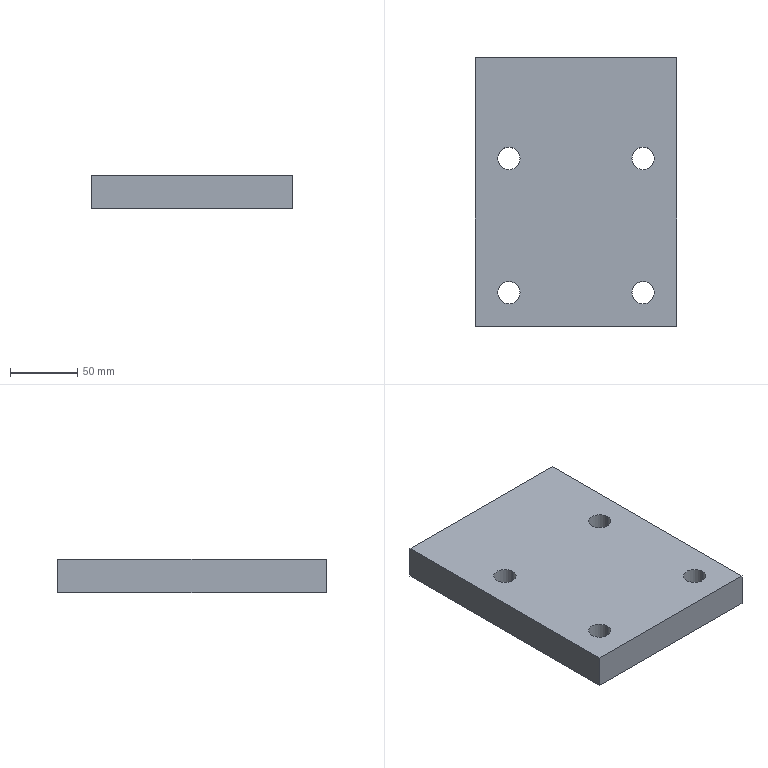Part | SolidWorks | features 3DProfileFeature 1, Extrusion 1, HoleWzd 1 | 1 solid | 14 faces | box 150 x 200 x 25 mm | volume 728181 mm3 | cylinder 8 | plane 6 | commonest cylinder face diameters 16.667 x8
STEP:
#1=CARTESIAN_POINT('',(16.666,125.,0.));
#2=VERTEX_POINT('',#1);
#3=CARTESIAN_POINT('',(33.334,125.,0.));
#4=VERTEX_POINT('',#3);
#5=CARTESIAN_POINT('',(25.,125.,0.));
#6=DIRECTION('',(0.,0.,1.));
#7=DIRECTION('',(1.,0.,0.));
#8=AXIS2_PLACEMENT_3D('',#5,#6,#7);
#9=CIRCLE('',#8,8.334);
#10=EDGE_CURVE('',#2,#4,#9,.T.);
#11=ORIENTED_EDGE('',*,*,#10,.F.);
#12=CARTESIAN_POINT('',(16.666,125.,25.));
#13=VERTEX_POINT('',#12);
#14=CARTESIAN_POINT('',(16.666,125.,25.));
#15=DIRECTION('',(0.,0.,1.));
#16=VECTOR('',#15,1000.);
#17=LINE('',#14,#16);
#18=EDGE_CURVE('',#2,#13,#17,.T.);
#19=ORIENTED_EDGE('',*,*,#18,.T.);
#20=CARTESIAN_POINT('',(33.334,125.,25.));
#21=VERTEX_POINT('',#20);
#22=CARTESIAN_POINT('',(25.,125.,25.));
#23=DIRECTION('',(0.,0.,1.));
#24=DIRECTION('',(1.,0.,0.));
#25=AXIS2_PLACEMENT_3D('',#22,#23,#24);
#26=CIRCLE('',#25,8.334);
#27=EDGE_CURVE('',#13,#21,#26,.T.);
#28=ORIENTED_EDGE('',*,*,#27,.T.);
#29=CARTESIAN_POINT('',(33.334,125.,25.));
#30=DIRECTION('',(0.,0.,1.));
#31=VECTOR('',#30,1000.);
#32=LINE('',#29,#31);
#33=EDGE_CURVE('',#4,#21,#32,.T.);
#34=ORIENTED_EDGE('',*,*,#33,.F.);
#35=EDGE_LOOP('',(#11,#19,#28,#34));
#36=FACE_OUTER_BOUND('',#35,.T.);
#37=CARTESIAN_POINT('',(25.,125.,25.));
#38=DIRECTION('',(0.,0.,1.));
#39=DIRECTION('',(1.,0.,0.));
#40=AXIS2_PLACEMENT_3D('',#37,#38,#39);
#41=CYLINDRICAL_SURFACE('',#40,8.334);
#42=ADVANCED_FACE('',(#36),#41,.F.);
#43=CARTESIAN_POINT('',(116.666,125.,0.));
#44=VERTEX_POINT('',#43);
#45=CARTESIAN_POINT('',(133.334,125.,0.));
#46=VERTEX_POINT('',#45);
#47=CARTESIAN_POINT('',(125.,125.,0.));
#48=DIRECTION('',(0.,0.,1.));
#49=DIRECTION('',(1.,0.,0.));
#50=AXIS2_PLACEMENT_3D('',#47,#48,#49);
#51=CIRCLE('',#50,8.334);
#52=EDGE_CURVE('',#44,#46,#51,.T.);
#53=ORIENTED_EDGE('',*,*,#52,.F.);
#54=CARTESIAN_POINT('',(116.666,125.,25.));
#55=VERTEX_POINT('',#54);
#56=CARTESIAN_POINT('',(116.666,125.,25.));
#57=DIRECTION('',(0.,0.,1.));
#58=VECTOR('',#57,1000.);
#59=LINE('',#56,#58);
#60=EDGE_CURVE('',#44,#55,#59,.T.);
#61=ORIENTED_EDGE('',*,*,#60,.T.);
#62=CARTESIAN_POINT('',(133.334,125.,25.));
#63=VERTEX_POINT('',#62);
#64=CARTESIAN_POINT('',(125.,125.,25.));
#65=DIRECTION('',(0.,0.,1.));
#66=DIRECTION('',(1.,0.,0.));
#67=AXIS2_PLACEMENT_3D('',#64,#65,#66);
#68=CIRCLE('',#67,8.334);
#69=EDGE_CURVE('',#55,#63,#68,.T.);
#70=ORIENTED_EDGE('',*,*,#69,.T.);
#71=CARTESIAN_POINT('',(133.334,125.,25.));
#72=DIRECTION('',(0.,0.,1.));
#73=VECTOR('',#72,1000.);
#74=LINE('',#71,#73);
#75=EDGE_CURVE('',#46,#63,#74,.T.);
#76=ORIENTED_EDGE('',*,*,#75,.F.);
#77=EDGE_LOOP('',(#53,#61,#70,#76));
#78=FACE_OUTER_BOUND('',#77,.T.);
#79=CARTESIAN_POINT('',(125.,125.,25.));
#80=DIRECTION('',(0.,0.,1.));
#81=DIRECTION('',(1.,0.,0.));
#82=AXIS2_PLACEMENT_3D('',#79,#80,#81);
#83=CYLINDRICAL_SURFACE('',#82,8.334);
#84=ADVANCED_FACE('',(#78),#83,.F.);
#85=CARTESIAN_POINT('',(16.666,25.,0.));
#86=VERTEX_POINT('',#85);
#87=CARTESIAN_POINT('',(33.334,25.,0.));
#88=VERTEX_POINT('',#87);
#89=CARTESIAN_POINT('',(25.,25.,0.));
#90=DIRECTION('',(0.,0.,1.));
#91=DIRECTION('',(1.,0.,0.));
#92=AXIS2_PLACEMENT_3D('',#89,#90,#91);
#93=CIRCLE('',#92,8.334);
#94=EDGE_CURVE('',#86,#88,#93,.T.);
#95=ORIENTED_EDGE('',*,*,#94,.F.);
#96=CARTESIAN_POINT('',(16.666,25.,25.));
#97=VERTEX_POINT('',#96);
#98=CARTESIAN_POINT('',(16.666,25.,25.));
#99=DIRECTION('',(0.,0.,1.));
#100=VECTOR('',#99,1000.);
#101=LINE('',#98,#100);
#102=EDGE_CURVE('',#86,#97,#101,.T.);
#103=ORIENTED_EDGE('',*,*,#102,.T.);
#104=CARTESIAN_POINT('',(33.334,25.,25.));
#105=VERTEX_POINT('',#104);
#106=CARTESIAN_POINT('',(25.,25.,25.));
#107=DIRECTION('',(0.,0.,1.));
#108=DIRECTION('',(1.,0.,0.));
#109=AXIS2_PLACEMENT_3D('',#106,#107,#108);
#110=CIRCLE('',#109,8.334);
#111=EDGE_CURVE('',#97,#105,#110,.T.);
#112=ORIENTED_EDGE('',*,*,#111,.T.);
#113=CARTESIAN_POINT('',(33.334,25.,25.));
#114=DIRECTION('',(0.,0.,1.));
#115=VECTOR('',#114,1000.);
#116=LINE('',#113,#115);
#117=EDGE_CURVE('',#88,#105,#116,.T.);
#118=ORIENTED_EDGE('',*,*,#117,.F.);
#119=EDGE_LOOP('',(#95,#103,#112,#118));
#120=FACE_OUTER_BOUND('',#119,.T.);
#121=CARTESIAN_POINT('',(25.,25.,25.));
#122=DIRECTION('',(0.,0.,1.));
#123=DIRECTION('',(1.,0.,0.));
#124=AXIS2_PLACEMENT_3D('',#121,#122,#123);
#125=CYLINDRICAL_SURFACE('',#124,8.334);
#126=ADVANCED_FACE('',(#120),#125,.F.);
#127=CARTESIAN_POINT('',(116.666,25.,0.));
#128=VERTEX_POINT('',#127);
#129=CARTESIAN_POINT('',(133.334,25.,0.));
#130=VERTEX_POINT('',#129);
#131=CARTESIAN_POINT('',(125.,25.,0.));
#132=DIRECTION('',(0.,0.,1.));
#133=DIRECTION('',(1.,0.,0.));
#134=AXIS2_PLACEMENT_3D('',#131,#132,#133);
#135=CIRCLE('',#134,8.334);
#136=EDGE_CURVE('',#128,#130,#135,.T.);
#137=ORIENTED_EDGE('',*,*,#136,.F.);
#138=CARTESIAN_POINT('',(116.666,25.,25.));
#139=VERTEX_POINT('',#138);
#140=CARTESIAN_POINT('',(116.666,25.,25.));
#141=DIRECTION('',(0.,0.,1.));
#142=VECTOR('',#141,1000.);
#143=LINE('',#140,#142);
#144=EDGE_CURVE('',#128,#139,#143,.T.);
#145=ORIENTED_EDGE('',*,*,#144,.T.);
#146=CARTESIAN_POINT('',(133.334,25.,25.));
#147=VERTEX_POINT('',#146);
#148=CARTESIAN_POINT('',(125.,25.,25.));
#149=DIRECTION('',(0.,0.,1.));
#150=DIRECTION('',(1.,0.,0.));
#151=AXIS2_PLACEMENT_3D('',#148,#149,#150);
#152=CIRCLE('',#151,8.334);
#153=EDGE_CURVE('',#139,#147,#152,.T.);
#154=ORIENTED_EDGE('',*,*,#153,.T.);
#155=CARTESIAN_POINT('',(133.334,25.,25.));
#156=DIRECTION('',(0.,0.,1.));
#157=VECTOR('',#156,1000.);
#158=LINE('',#155,#157);
#159=EDGE_CURVE('',#130,#147,#158,.T.);
#160=ORIENTED_EDGE('',*,*,#159,.F.);
#161=EDGE_LOOP('',(#137,#145,#154,#160));
#162=FACE_OUTER_BOUND('',#161,.T.);
#163=CARTESIAN_POINT('',(125.,25.,25.));
#164=DIRECTION('',(0.,0.,1.));
#165=DIRECTION('',(1.,0.,0.));
#166=AXIS2_PLACEMENT_3D('',#163,#164,#165);
#167=CYLINDRICAL_SURFACE('',#166,8.334);
#168=ADVANCED_FACE('',(#162),#167,.F.);
#169=CARTESIAN_POINT('',(25.,125.,0.));
#170=DIRECTION('',(0.,0.,1.));
#171=DIRECTION('',(1.,0.,0.));
#172=AXIS2_PLACEMENT_3D('',#169,#170,#171);
#173=CIRCLE('',#172,8.334);
#174=EDGE_CURVE('',#4,#2,#173,.T.);
#175=ORIENTED_EDGE('',*,*,#174,.T.);
#176=ORIENTED_EDGE('',*,*,#10,.T.);
#177=EDGE_LOOP('',(#175,#176));
#178=FACE_BOUND('',#177,.T.);
#179=CARTESIAN_POINT('',(125.,125.,0.));
#180=DIRECTION('',(0.,0.,1.));
#181=DIRECTION('',(1.,0.,0.));
#182=AXIS2_PLACEMENT_3D('',#179,#180,#181);
#183=CIRCLE('',#182,8.334);
#184=EDGE_CURVE('',#46,#44,#183,.T.);
#185=ORIENTED_EDGE('',*,*,#184,.T.);
#186=ORIENTED_EDGE('',*,*,#52,.T.);
#187=EDGE_LOOP('',(#185,#186));
#188=FACE_BOUND('',#187,.T.);
#189=CARTESIAN_POINT('',(0.,200.,0.));
#190=VERTEX_POINT('',#189);
#191=CARTESIAN_POINT('',(0.,0.,0.));
#192=VERTEX_POINT('',#191);
#193=CARTESIAN_POINT('',(0.,0.,0.));
#194=DIRECTION('',(0.,-1.,0.));
#195=VECTOR('',#194,1000.);
#196=LINE('',#193,#195);
#197=EDGE_CURVE('',#190,#192,#196,.T.);
#198=ORIENTED_EDGE('',*,*,#197,.F.);
#199=CARTESIAN_POINT('',(150.,200.,0.));
#200=VERTEX_POINT('',#199);
#201=CARTESIAN_POINT('',(0.,200.,0.));
#202=DIRECTION('',(-1.,0.,0.));
#203=VECTOR('',#202,1000.);
#204=LINE('',#201,#203);
#205=EDGE_CURVE('',#200,#190,#204,.T.);
#206=ORIENTED_EDGE('',*,*,#205,.F.);
#207=CARTESIAN_POINT('',(150.,0.,0.));
#208=VERTEX_POINT('',#207);
#209=CARTESIAN_POINT('',(150.,0.,0.));
#210=DIRECTION('',(0.,1.,0.));
#211=VECTOR('',#210,1000.);
#212=LINE('',#209,#211);
#213=EDGE_CURVE('',#208,#200,#212,.T.);
#214=ORIENTED_EDGE('',*,*,#213,.F.);
#215=CARTESIAN_POINT('',(0.,0.,0.));
#216=DIRECTION('',(1.,0.,0.));
#217=VECTOR('',#216,1000.);
#218=LINE('',#215,#217);
#219=EDGE_CURVE('',#192,#208,#218,.T.);
#220=ORIENTED_EDGE('',*,*,#219,.F.);
#221=EDGE_LOOP('',(#198,#206,#214,#220));
#222=FACE_OUTER_BOUND('',#221,.T.);
#223=CARTESIAN_POINT('',(125.,25.,0.));
#224=DIRECTION('',(0.,0.,1.));
#225=DIRECTION('',(1.,0.,0.));
#226=AXIS2_PLACEMENT_3D('',#223,#224,#225);
#227=CIRCLE('',#226,8.334);
#228=EDGE_CURVE('',#130,#128,#227,.T.);
#229=ORIENTED_EDGE('',*,*,#228,.T.);
#230=ORIENTED_EDGE('',*,*,#136,.T.);
#231=EDGE_LOOP('',(#229,#230));
#232=FACE_BOUND('',#231,.T.);
#233=CARTESIAN_POINT('',(25.,25.,0.));
#234=DIRECTION('',(0.,0.,1.));
#235=DIRECTION('',(1.,0.,0.));
#236=AXIS2_PLACEMENT_3D('',#233,#234,#235);
#237=CIRCLE('',#236,8.334);
#238=EDGE_CURVE('',#88,#86,#237,.T.);
#239=ORIENTED_EDGE('',*,*,#238,.T.);
#240=ORIENTED_EDGE('',*,*,#94,.T.);
#241=EDGE_LOOP('',(#239,#240));
#242=FACE_BOUND('',#241,.T.);
#243=CARTESIAN_POINT('',(0.,0.,0.));
#244=DIRECTION('',(0.,0.,-1.));
#245=DIRECTION('',(-1.,0.,0.));
#246=AXIS2_PLACEMENT_3D('',#243,#244,#245);
#247=PLANE('',#246);
#248=ADVANCED_FACE('',(#178,#188,#222,#232,#242),#247,.T.);
#249=ORIENTED_EDGE('',*,*,#197,.T.);
#250=CARTESIAN_POINT('',(0.,0.,25.));
#251=VERTEX_POINT('',#250);
#252=CARTESIAN_POINT('',(0.,0.,25.));
#253=DIRECTION('',(0.,0.,-1.));
#254=VECTOR('',#253,1000.);
#255=LINE('',#252,#254);
#256=EDGE_CURVE('',#251,#192,#255,.T.);
#257=ORIENTED_EDGE('',*,*,#256,.F.);
#258=CARTESIAN_POINT('',(0.,200.,25.));
#259=VERTEX_POINT('',#258);
#260=CARTESIAN_POINT('',(0.,0.,25.));
#261=DIRECTION('',(0.,-1.,0.));
#262=VECTOR('',#261,1000.);
#263=LINE('',#260,#262);
#264=EDGE_CURVE('',#259,#251,#263,.T.);
#265=ORIENTED_EDGE('',*,*,#264,.F.);
#266=CARTESIAN_POINT('',(0.,200.,25.));
#267=DIRECTION('',(0.,0.,-1.));
#268=VECTOR('',#267,1000.);
#269=LINE('',#266,#268);
#270=EDGE_CURVE('',#259,#190,#269,.T.);
#271=ORIENTED_EDGE('',*,*,#270,.T.);
#272=EDGE_LOOP('',(#249,#257,#265,#271));
#273=FACE_OUTER_BOUND('',#272,.T.);
#274=CARTESIAN_POINT('',(0.,0.,25.));
#275=DIRECTION('',(1.,0.,0.));
#276=DIRECTION('',(0.,1.,0.));
#277=AXIS2_PLACEMENT_3D('',#274,#275,#276);
#278=PLANE('',#277);
#279=ADVANCED_FACE('',(#273),#278,.F.);
#280=ORIENTED_EDGE('',*,*,#219,.T.);
#281=CARTESIAN_POINT('',(150.,0.,25.));
#282=VERTEX_POINT('',#281);
#283=CARTESIAN_POINT('',(150.,0.,25.));
#284=DIRECTION('',(0.,0.,-1.));
#285=VECTOR('',#284,1000.);
#286=LINE('',#283,#285);
#287=EDGE_CURVE('',#282,#208,#286,.T.);
#288=ORIENTED_EDGE('',*,*,#287,.F.);
#289=CARTESIAN_POINT('',(0.,0.,25.));
#290=DIRECTION('',(1.,0.,0.));
#291=VECTOR('',#290,1000.);
#292=LINE('',#289,#291);
#293=EDGE_CURVE('',#251,#282,#292,.T.);
#294=ORIENTED_EDGE('',*,*,#293,.F.);
#295=ORIENTED_EDGE('',*,*,#256,.T.);
#296=EDGE_LOOP('',(#280,#288,#294,#295));
#297=FACE_OUTER_BOUND('',#296,.T.);
#298=CARTESIAN_POINT('',(0.,0.,25.));
#299=DIRECTION('',(0.,1.,0.));
#300=DIRECTION('',(0.,0.,1.));
#301=AXIS2_PLACEMENT_3D('',#298,#299,#300);
#302=PLANE('',#301);
#303=ADVANCED_FACE('',(#297),#302,.F.);
#304=ORIENTED_EDGE('',*,*,#213,.T.);
#305=CARTESIAN_POINT('',(150.,200.,25.));
#306=VERTEX_POINT('',#305);
#307=CARTESIAN_POINT('',(150.,200.,25.));
#308=DIRECTION('',(0.,0.,-1.));
#309=VECTOR('',#308,1000.);
#310=LINE('',#307,#309);
#311=EDGE_CURVE('',#306,#200,#310,.T.);
#312=ORIENTED_EDGE('',*,*,#311,.F.);
#313=CARTESIAN_POINT('',(150.,0.,25.));
#314=DIRECTION('',(0.,1.,0.));
#315=VECTOR('',#314,1000.);
#316=LINE('',#313,#315);
#317=EDGE_CURVE('',#282,#306,#316,.T.);
#318=ORIENTED_EDGE('',*,*,#317,.F.);
#319=ORIENTED_EDGE('',*,*,#287,.T.);
#320=EDGE_LOOP('',(#304,#312,#318,#319));
#321=FACE_OUTER_BOUND('',#320,.T.);
#322=CARTESIAN_POINT('',(150.,0.,25.));
#323=DIRECTION('',(-1.,0.,0.));
#324=DIRECTION('',(0.,0.,1.));
#325=AXIS2_PLACEMENT_3D('',#322,#323,#324);
#326=PLANE('',#325);
#327=ADVANCED_FACE('',(#321),#326,.F.);
#328=ORIENTED_EDGE('',*,*,#205,.T.);
#329=ORIENTED_EDGE('',*,*,#270,.F.);
#330=CARTESIAN_POINT('',(0.,200.,25.));
#331=DIRECTION('',(-1.,0.,0.));
#332=VECTOR('',#331,1000.);
#333=LINE('',#330,#332);
#334=EDGE_CURVE('',#306,#259,#333,.T.);
#335=ORIENTED_EDGE('',*,*,#334,.F.);
#336=ORIENTED_EDGE('',*,*,#311,.T.);
#337=EDGE_LOOP('',(#328,#329,#335,#336));
#338=FACE_OUTER_BOUND('',#337,.T.);
#339=CARTESIAN_POINT('',(0.,200.,25.));
#340=DIRECTION('',(0.,-1.,0.));
#341=DIRECTION('',(1.,0.,0.));
#342=AXIS2_PLACEMENT_3D('',#339,#340,#341);
#343=PLANE('',#342);
#344=ADVANCED_FACE('',(#338),#343,.F.);
#345=CARTESIAN_POINT('',(25.,125.,25.));
#346=DIRECTION('',(0.,0.,1.));
#347=DIRECTION('',(1.,0.,0.));
#348=AXIS2_PLACEMENT_3D('',#345,#346,#347);
#349=CIRCLE('',#348,8.334);
#350=EDGE_CURVE('',#21,#13,#349,.T.);
#351=ORIENTED_EDGE('',*,*,#350,.F.);
#352=ORIENTED_EDGE('',*,*,#27,.F.);
#353=EDGE_LOOP('',(#351,#352));
#354=FACE_BOUND('',#353,.T.);
#355=CARTESIAN_POINT('',(125.,125.,25.));
#356=DIRECTION('',(0.,0.,1.));
#357=DIRECTION('',(1.,0.,0.));
#358=AXIS2_PLACEMENT_3D('',#355,#356,#357);
#359=CIRCLE('',#358,8.334);
#360=EDGE_CURVE('',#63,#55,#359,.T.);
#361=ORIENTED_EDGE('',*,*,#360,.F.);
#362=ORIENTED_EDGE('',*,*,#69,.F.);
#363=EDGE_LOOP('',(#361,#362));
#364=FACE_BOUND('',#363,.T.);
#365=CARTESIAN_POINT('',(25.,25.,25.));
#366=DIRECTION('',(0.,0.,1.));
#367=DIRECTION('',(1.,0.,0.));
#368=AXIS2_PLACEMENT_3D('',#365,#366,#367);
#369=CIRCLE('',#368,8.334);
#370=EDGE_CURVE('',#105,#97,#369,.T.);
#371=ORIENTED_EDGE('',*,*,#370,.F.);
#372=ORIENTED_EDGE('',*,*,#111,.F.);
#373=EDGE_LOOP('',(#371,#372));
#374=FACE_BOUND('',#373,.T.);
#375=CARTESIAN_POINT('',(125.,25.,25.));
#376=DIRECTION('',(0.,0.,1.));
#377=DIRECTION('',(1.,0.,0.));
#378=AXIS2_PLACEMENT_3D('',#375,#376,#377);
#379=CIRCLE('',#378,8.334);
#380=EDGE_CURVE('',#147,#139,#379,.T.);
#381=ORIENTED_EDGE('',*,*,#380,.F.);
#382=ORIENTED_EDGE('',*,*,#153,.F.);
#383=EDGE_LOOP('',(#381,#382));
#384=FACE_BOUND('',#383,.T.);
#385=ORIENTED_EDGE('',*,*,#264,.T.);
#386=ORIENTED_EDGE('',*,*,#293,.T.);
#387=ORIENTED_EDGE('',*,*,#317,.T.);
#388=ORIENTED_EDGE('',*,*,#334,.T.);
#389=EDGE_LOOP('',(#385,#386,#387,#388));
#390=FACE_OUTER_BOUND('',#389,.T.);
#391=CARTESIAN_POINT('',(0.,0.,25.));
#392=DIRECTION('',(0.,0.,-1.));
#393=DIRECTION('',(-1.,0.,0.));
#394=AXIS2_PLACEMENT_3D('',#391,#392,#393);
#395=PLANE('',#394);
#396=ADVANCED_FACE('',(#354,#364,#374,#384,#390),#395,.F.);
#397=ORIENTED_EDGE('',*,*,#144,.F.);
#398=ORIENTED_EDGE('',*,*,#228,.F.);
#399=ORIENTED_EDGE('',*,*,#159,.T.);
#400=ORIENTED_EDGE('',*,*,#380,.T.);
#401=EDGE_LOOP('',(#397,#398,#399,#400));
#402=FACE_OUTER_BOUND('',#401,.T.);
#403=CARTESIAN_POINT('',(125.,25.,25.));
#404=DIRECTION('',(0.,0.,1.));
#405=DIRECTION('',(1.,0.,0.));
#406=AXIS2_PLACEMENT_3D('',#403,#404,#405);
#407=CYLINDRICAL_SURFACE('',#406,8.334);
#408=ADVANCED_FACE('',(#402),#407,.F.);
#409=ORIENTED_EDGE('',*,*,#102,.F.);
#410=ORIENTED_EDGE('',*,*,#238,.F.);
#411=ORIENTED_EDGE('',*,*,#117,.T.);
#412=ORIENTED_EDGE('',*,*,#370,.T.);
#413=EDGE_LOOP('',(#409,#410,#411,#412));
#414=FACE_OUTER_BOUND('',#413,.T.);
#415=CARTESIAN_POINT('',(25.,25.,25.));
#416=DIRECTION('',(0.,0.,1.));
#417=DIRECTION('',(1.,0.,0.));
#418=AXIS2_PLACEMENT_3D('',#415,#416,#417);
#419=CYLINDRICAL_SURFACE('',#418,8.334);
#420=ADVANCED_FACE('',(#414),#419,.F.);
#421=ORIENTED_EDGE('',*,*,#60,.F.);
#422=ORIENTED_EDGE('',*,*,#184,.F.);
#423=ORIENTED_EDGE('',*,*,#75,.T.);
#424=ORIENTED_EDGE('',*,*,#360,.T.);
#425=EDGE_LOOP('',(#421,#422,#423,#424));
#426=FACE_OUTER_BOUND('',#425,.T.);
#427=CARTESIAN_POINT('',(125.,125.,25.));
#428=DIRECTION('',(0.,0.,1.));
#429=DIRECTION('',(1.,0.,0.));
#430=AXIS2_PLACEMENT_3D('',#427,#428,#429);
#431=CYLINDRICAL_SURFACE('',#430,8.334);
#432=ADVANCED_FACE('',(#426),#431,.F.);
#433=ORIENTED_EDGE('',*,*,#18,.F.);
#434=ORIENTED_EDGE('',*,*,#174,.F.);
#435=ORIENTED_EDGE('',*,*,#33,.T.);
#436=ORIENTED_EDGE('',*,*,#350,.T.);
#437=EDGE_LOOP('',(#433,#434,#435,#436));
#438=FACE_OUTER_BOUND('',#437,.T.);
#439=CARTESIAN_POINT('',(25.,125.,25.));
#440=DIRECTION('',(0.,0.,1.));
#441=DIRECTION('',(1.,0.,0.));
#442=AXIS2_PLACEMENT_3D('',#439,#440,#441);
#443=CYLINDRICAL_SURFACE('',#442,8.334);
#444=ADVANCED_FACE('',(#438),#443,.F.);
#445=CLOSED_SHELL('',(#42,#84,#126,#168,#248,#279,#303,#327,#344,#396,#408,#420,#432,#444));
#446=MANIFOLD_SOLID_BREP('',#445);
#447=CARTESIAN_POINT('',(0.,0.,0.));
#448=DIRECTION('',(0.,0.,1.));
#449=DIRECTION('',(1.,0.,0.));
#450=AXIS2_PLACEMENT_3D('',#447,#448,#449);
#451=(LENGTH_UNIT()NAMED_UNIT(*)SI_UNIT(.MILLI.,.METRE.));
#452=UNCERTAINTY_MEASURE_WITH_UNIT(LENGTH_MEASURE(0.00001),#451,'','');
#453=(NAMED_UNIT(*)PLANE_ANGLE_UNIT()SI_UNIT($,.RADIAN.));
#454=(NAMED_UNIT(*)SI_UNIT($,.STERADIAN.)SOLID_ANGLE_UNIT());
#455=(GEOMETRIC_REPRESENTATION_CONTEXT(3)GLOBAL_UNCERTAINTY_ASSIGNED_CONTEXT((#452))GLOBAL_UNIT_ASSIGNED_CONTEXT((#451,#453,#454))REPRESENTATION_CONTEXT('',''));
#456=ADVANCED_BREP_SHAPE_REPRESENTATION('',(#446,#450),#455);